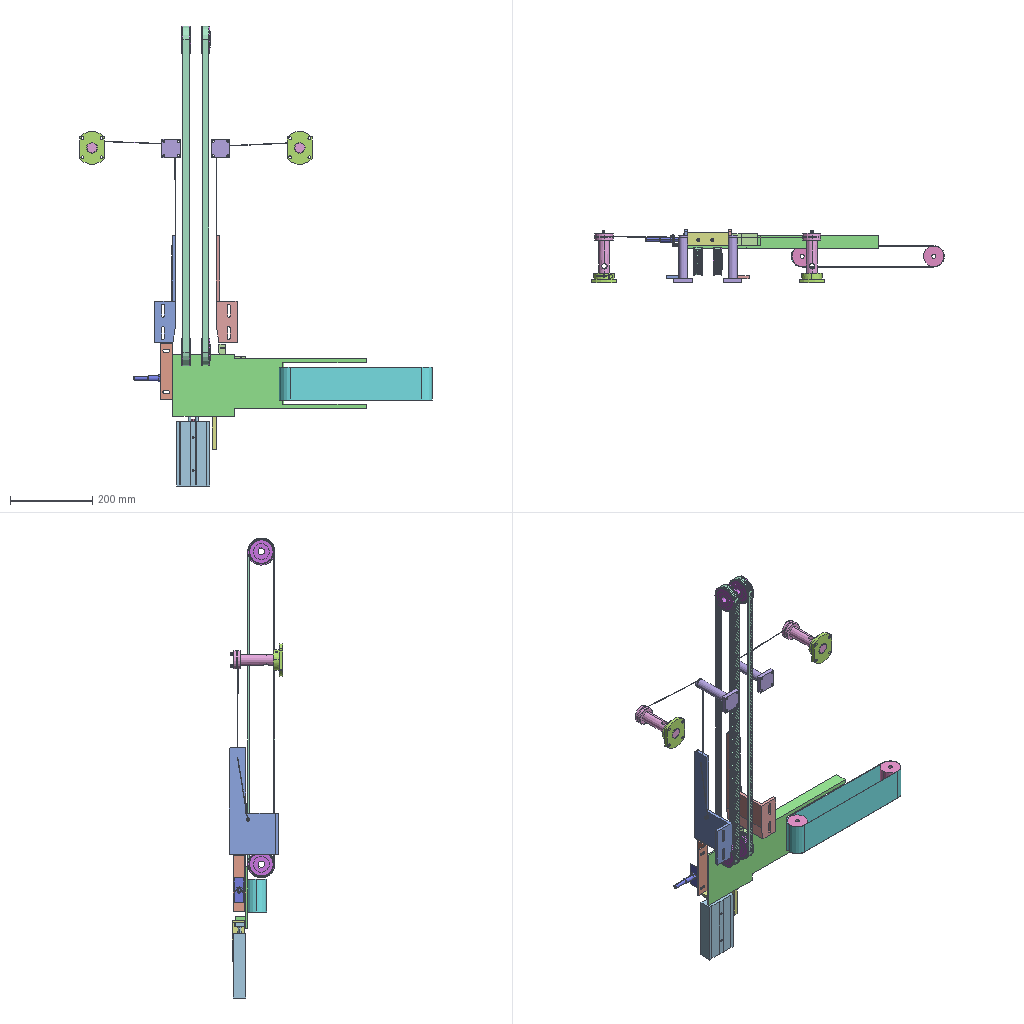Assembly | SolidWorks | 20 different items | 29 placed | box 857 x 130 x 1118 mm
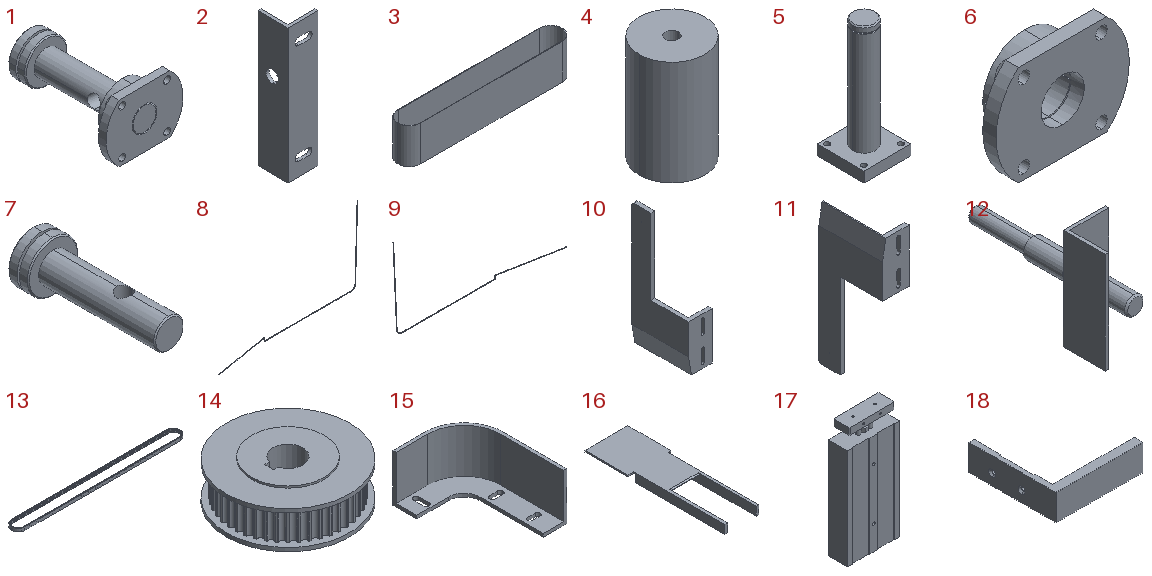Parts list (item | name | quantity | parent item | size | volume | features):
1 | (subassembly) | x2 | - | 80 x 126 x 60 mm | 124999 mm3 | -
2 | - | x1 | - | 30 x 30 x 135 mm | 22072 mm3 | features ICE 2, Extrusion 1
3 | - | x1 | - | 372 x 52 x 80 mm | 64018 mm3 | features Extrusion 1
4 | - | x2 | - | 50 x 50 x 80 mm | 150796 mm3 | features Extrusion 1
5 | - | x2 | - | 45 x 45 x 115 mm | 59266 mm3 | features ICE 2, Chamfer 1, Extrusion 1
6 | - | x2 | in 1 | 80 x 23 x 60 mm | 48901 mm3 | features ICE 6, 3DProfileFeature 1, HoleWzd 1, Revolution 1
7 | - | x2 | in 1 | 44 x 120 x 44 mm | 75501 mm3 | features 3DProfileFeature 1, Chamfer 1, CirPattern 1, HoleWzd 1, ICE 1, Revolution 1
8 | - | x1 | - | 405.14 x 27.994 x 201.874 mm | 473.079 mm3 | features 3DProfileFeature 4, Sweep 1
9 | - | x1 | - | 401.907 x 29.216 x 204.55 mm | 473.935 mm3 | features 3DProfileFeature 4, Sweep 1
10 | - | x1 | - | 50 x 120 x 260 mm | 164749 mm3 | features ICE 4, 3DProfileFeature 1, Extrusion 1, Fillet 1, HoleWzd 1
11 | - | x1 | - | 50 x 120 x 260 mm | 164749 mm3 | features ICE 4, 3DProfileFeature 1, Extrusion 1, Fillet 1, HoleWzd 1
12 | - | x1 | - | 25 x 95 x 60 mm | 14738 mm3 | features ICE 4, Chamfer 1, ExtruThin 1
13 | - | x2 | - | 825 x 65 x 15 mm | 85490 mm3 | features CurvePattern 3, ICE 3, Extrusion 1
14 | - | x4 | - | 66 x 66 x 22 mm | 54187 mm3 | features ICE 6, CirPattern 1, Extrusion 1, Fillet 1
15 | - | x1 | - | 45 x 65 x 30 mm | 7932 mm3 | features ICE 2, ExtruThin 1
16 | - | x1 | - | 150 x 470 x 30 mm | 353727 mm3 | features Chamfer 1, Extrusion 1, ICE 1
17 | - | x1 | - | 81 x 30 x 183 mm | 382969 mm3 | features Boss 4, HoleWzd 3, Extrusion 1
18 | - | x1 | - | 100 x 100 x 30 mm | 45451 mm3 | features ICE 2, Chamfer 1, Extrusion 1
19 | hexagon socket countersunk head screws gb | x1 | - | - | - | -
20 | hexagon socket head cap screws gb | x1 | - | - | - | -
Mates (type | each side: item.copy, entity, surface, feature):
In the top assembly
Coincident | 10.1 face plane Boss-Extrude1 | 11.1 face plane Boss-Extrude1 | 2 times
DistanceDim | 11.1 face plane Boss-Extrude1 | 10.1 face plane Boss-Extrude1
Coincident | 6.1 face plane Revolve1 | 5.1 face plane Boss-Extrude1
Coincident | 10.1 face plane Cut-Extrude1 | 16.1 face plane Boss-Extrude1
DistanceDim | 16.1 face plane Boss-Extrude1 | 10.1 face plane Boss-Extrude1
Coincident | 11.1 edge | 16.1 face plane Boss-Extrude1
Coincident | 16.1 face plane Boss-Extrude1 | 17.1 face plane Extrude1
DistanceDim | 17.1 face plane Extrude1 | 11.1 face plane Boss-Extrude1
Coincident | 17.1 face plane Extrude3 | 18.1 face plane Boss-Extrude1 | 2 times
Coincident | 10.1 face plane Boss-Extrude1 | 18.1 face plane Boss-Extrude1
Coincident | 16.1 face plane Boss-Extrude1 | 18.1 face plane Boss-Extrude1
DistanceDim | 5.1 face plane Boss-Extrude2 | 10.1 face plane Boss-Extrude1
Tangent | 10.1 face plane Boss-Extrude1 | 5.1 face cylinder Cut-Extrude1
DistanceDim | 5.1 face cylinder Boss-Extrude2 | 10.1 face plane Boss-Extrude1
Parallel | 10.1 face plane Boss-Extrude1 | 5.1 face plane Boss-Extrude1
DistanceDim | 6.1 face plane Cut-Extrude1 | 5.1 face plane Boss-Extrude1
DistanceDim | 7.1 face cylinder Revolve1 | 10.1 face plane Boss-Extrude1
DistanceDim | 14.1 face plane Boss-Extrude4 | 11.1 face plane Boss-Extrude1
DistanceDim | 14.2 face plane Boss-Extrude5 | 10.1 face plane Boss-Extrude1
Concentric | 14.1 face cylinder Cut-Extrude2 | 14.2 face cylinder Cut-Extrude2
Tangent | 14.1 face cylinder Boss-Extrude2 | 16.1 face plane Boss-Extrude1
DistanceDim | 14.2 face cylinder Cut-Extrude2 | 10.1 face plane Boss-Extrude1
Coincident | 5.2 face plane Boss-Extrude1 | 6.2 face plane Revolve1
Coincident | 5.1 face plane Boss-Extrude1 | 5.2 face plane Boss-Extrude1 | 2 times
Tangent | 11.1 face plane Boss-Extrude1 | 5.2 face cylinder Cut-Extrude1
DistanceDim | 11.1 face plane Boss-Extrude1 | 7.2 face cylinder Revolve1
DistanceDim | 5.2 face plane Boss-Extrude1 | 6.2 face plane Cut-Extrude1
Coincident | 14.2 face plane Boss-Extrude5 | 14.3 face plane Boss-Extrude5
Coincident | 14.1 face plane Boss-Extrude5 | 14.4 face plane Boss-Extrude4
Concentric | 14.4 face cylinder Cut-Extrude2 | 14.3 face cylinder Cut-Extrude2
Tangent | 16.1 face plane Boss-Extrude1 | 14.3 face cylinder Boss-Extrude3
DistanceDim | 14.3 face cylinder Cut-Extrude2 | 14.2 face cylinder Cut-Extrude2
Concentric | 14.3 face cylinder Boss-Extrude3 | 13.1 face cylinder Boss-Extrude1
DistanceDim | 13.1 face plane Boss-Extrude1 | 14.4 face plane Boss-Extrude2
Parallel | 16.1 face plane Boss-Extrude1 | 13.1 face plane Boss-Extrude1
Coincident | 13.1 face plane Boss-Extrude1 | 13.2 face plane Boss-Extrude1
DistanceDim | 13.2 face plane Boss-Extrude1 | 14.3 face plane Boss-Extrude3
Concentric | 14.3 face cylinder Boss-Extrude2 | 13.2 face cylinder Boss-Extrude1
Coincident | 16.1 face plane Boss-Extrude1 | 2.1 face plane Boss-Extrude1 | 2 times
DistanceDim | 2.1 face plane Boss-Extrude1 | 11.1 face plane Boss-Extrude1
Coincident | 2.1 face plane Boss-Extrude1 | 12.1 face plane Boss-Extrude3
Coincident | 2.1 face plane Boss-Extrude1 | 12.1 face plane Extrude-Thin1
Coincident | 16.1 face plane Boss-Extrude1 | 15.1 face plane Extrude-Thin1
Coincident | 16.1 face plane Boss-Extrude2 | 15.1 face plane Extrude-Thin1
Coincident | 10.1 edge | 15.1 face plane Extrude-Thin1
Coincident | 4.1 face plane Boss-Extrude1 | 4.2 face plane Boss-Extrude1
Tangent | 16.1 face plane Boss-Extrude1 | 4.1 face cylinder Boss-Extrude1
DistanceDim | 4.1 face plane Boss-Extrude1 | 16.1 face plane Boss-Extrude2
Tangent | 16.1 face plane Boss-Extrude1 | 4.2 face cylinder Boss-Extrude1
DistanceDim | 4.1 face cylinder Boss-Extrude1 | 4.2 face cylinder Boss-Extrude1
DistanceDim | 4.1 face cylinder Boss-Extrude1 | 16.1 face plane Boss-Extrude1
Concentric | 4.2 face cylinder Boss-Extrude1 | 3.1 face cylinder Boss-Extrude1
Coincident | 4.2 edge | 3.1 face plane Boss-Extrude1
Parallel | 16.1 face plane Boss-Extrude1 | 3.1 face plane Boss-Extrude1
InPlace | 10.1 face plane Boss-Extrude1 | 9.1 plane
InPlace | 11.1 face plane Boss-Extrude1 | 8.1 plane
In subassembly 1
Concentric | 6.3 face cylinder Revolve1 | 7.3 face cylinder Revolve1
Coincident | 6.3 face plane Revolve1 | 7.3 face plane Revolve1